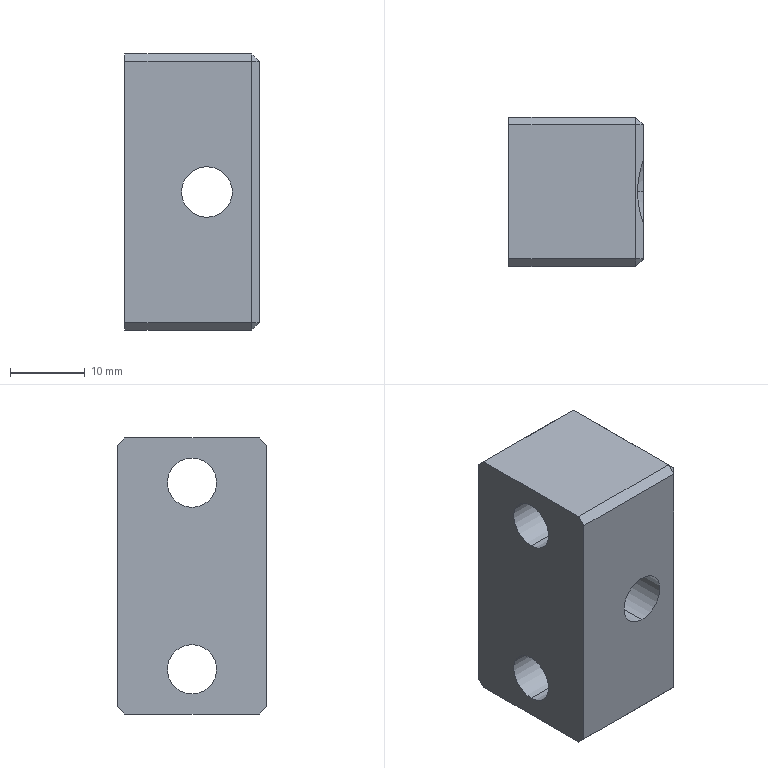Part | SolidWorks | features BaseBody 1 | 1 solid | 34 faces | box 18 x 20 x 37 mm | volume 9780 mm3 | plane 20 | cylinder 10 | cone 4 | commonest cylinder face diameters 6.6 x4 11 x4 6.8 x2
STEP:
#1=CARTESIAN_POINT('',(104.247,1826.,-338.8));
#2=VERTEX_POINT('',#1);
#3=CARTESIAN_POINT('',(104.247,1826.,-332.2));
#4=VERTEX_POINT('',#3);
#5=CARTESIAN_POINT('',(104.247,1826.,-335.5));
#6=DIRECTION('',(-1.,0.,0.));
#7=DIRECTION('',(0.,0.,-1.));
#8=AXIS2_PLACEMENT_3D('',#5,#6,#7);
#9=CIRCLE('',#8,3.3);
#10=EDGE_CURVE('',#2,#4,#9,.T.);
#11=ORIENTED_EDGE('',*,*,#10,.T.);
#12=CARTESIAN_POINT('',(110.247,1826.,-332.2));
#13=VERTEX_POINT('',#12);
#14=CARTESIAN_POINT('',(122.247,1826.,-332.2));
#15=DIRECTION('',(1.,0.,0.));
#16=VECTOR('',#15,1000.);
#17=LINE('',#14,#16);
#18=EDGE_CURVE('',#4,#13,#17,.T.);
#19=ORIENTED_EDGE('',*,*,#18,.T.);
#20=CARTESIAN_POINT('',(110.247,1826.,-338.8));
#21=VERTEX_POINT('',#20);
#22=CARTESIAN_POINT('',(110.247,1826.,-335.5));
#23=DIRECTION('',(-1.,0.,0.));
#24=DIRECTION('',(0.,0.,-1.));
#25=AXIS2_PLACEMENT_3D('',#22,#23,#24);
#26=CIRCLE('',#25,3.3);
#27=EDGE_CURVE('',#21,#13,#26,.T.);
#28=ORIENTED_EDGE('',*,*,#27,.F.);
#29=CARTESIAN_POINT('',(122.247,1826.,-338.8));
#30=DIRECTION('',(1.,0.,0.));
#31=VECTOR('',#30,1000.);
#32=LINE('',#29,#31);
#33=EDGE_CURVE('',#2,#21,#32,.T.);
#34=ORIENTED_EDGE('',*,*,#33,.F.);
#35=EDGE_LOOP('',(#11,#19,#28,#34));
#36=FACE_OUTER_BOUND('',#35,.T.);
#37=CARTESIAN_POINT('',(122.247,1826.,-335.5));
#38=DIRECTION('',(1.,0.,0.));
#39=DIRECTION('',(0.,0.,-1.));
#40=AXIS2_PLACEMENT_3D('',#37,#38,#39);
#41=CYLINDRICAL_SURFACE('',#40,3.3);
#42=ADVANCED_FACE('',(#36),#41,.F.);
#43=CARTESIAN_POINT('',(104.247,1826.,-363.8));
#44=VERTEX_POINT('',#43);
#45=CARTESIAN_POINT('',(104.247,1826.,-357.2));
#46=VERTEX_POINT('',#45);
#47=CARTESIAN_POINT('',(104.247,1826.,-360.5));
#48=DIRECTION('',(-1.,0.,0.));
#49=DIRECTION('',(0.,0.,-1.));
#50=AXIS2_PLACEMENT_3D('',#47,#48,#49);
#51=CIRCLE('',#50,3.3);
#52=EDGE_CURVE('',#44,#46,#51,.T.);
#53=ORIENTED_EDGE('',*,*,#52,.T.);
#54=CARTESIAN_POINT('',(110.247,1826.,-357.2));
#55=VERTEX_POINT('',#54);
#56=CARTESIAN_POINT('',(122.247,1826.,-357.2));
#57=DIRECTION('',(1.,0.,0.));
#58=VECTOR('',#57,1000.);
#59=LINE('',#56,#58);
#60=EDGE_CURVE('',#46,#55,#59,.T.);
#61=ORIENTED_EDGE('',*,*,#60,.T.);
#62=CARTESIAN_POINT('',(110.247,1826.,-363.8));
#63=VERTEX_POINT('',#62);
#64=CARTESIAN_POINT('',(110.247,1826.,-360.5));
#65=DIRECTION('',(-1.,0.,0.));
#66=DIRECTION('',(0.,0.,-1.));
#67=AXIS2_PLACEMENT_3D('',#64,#65,#66);
#68=CIRCLE('',#67,3.3);
#69=EDGE_CURVE('',#63,#55,#68,.T.);
#70=ORIENTED_EDGE('',*,*,#69,.F.);
#71=CARTESIAN_POINT('',(122.247,1826.,-363.8));
#72=DIRECTION('',(1.,0.,0.));
#73=VECTOR('',#72,1000.);
#74=LINE('',#71,#73);
#75=EDGE_CURVE('',#44,#63,#74,.T.);
#76=ORIENTED_EDGE('',*,*,#75,.F.);
#77=EDGE_LOOP('',(#53,#61,#70,#76));
#78=FACE_OUTER_BOUND('',#77,.T.);
#79=CARTESIAN_POINT('',(122.247,1826.,-360.5));
#80=DIRECTION('',(1.,0.,0.));
#81=DIRECTION('',(0.,0.,-1.));
#82=AXIS2_PLACEMENT_3D('',#79,#80,#81);
#83=CYLINDRICAL_SURFACE('',#82,3.3);
#84=ADVANCED_FACE('',(#78),#83,.F.);
#85=CARTESIAN_POINT('',(115.247,1836.,-351.4));
#86=VERTEX_POINT('',#85);
#87=CARTESIAN_POINT('',(115.247,1836.,-344.6));
#88=VERTEX_POINT('',#87);
#89=CARTESIAN_POINT('',(115.247,1836.,-348.));
#90=DIRECTION('',(0.,1.,0.));
#91=DIRECTION('',(0.,0.,-1.));
#92=AXIS2_PLACEMENT_3D('',#89,#90,#91);
#93=CIRCLE('',#92,3.4);
#94=EDGE_CURVE('',#86,#88,#93,.T.);
#95=ORIENTED_EDGE('',*,*,#94,.T.);
#96=CARTESIAN_POINT('',(115.247,1816.,-344.6));
#97=VERTEX_POINT('',#96);
#98=CARTESIAN_POINT('',(115.247,1816.,-344.6));
#99=DIRECTION('',(0.,-1.,0.));
#100=VECTOR('',#99,1000.);
#101=LINE('',#98,#100);
#102=EDGE_CURVE('',#88,#97,#101,.T.);
#103=ORIENTED_EDGE('',*,*,#102,.T.);
#104=CARTESIAN_POINT('',(115.247,1816.,-351.4));
#105=VERTEX_POINT('',#104);
#106=CARTESIAN_POINT('',(115.247,1816.,-348.));
#107=DIRECTION('',(0.,-1.,0.));
#108=DIRECTION('',(0.,0.,-1.));
#109=AXIS2_PLACEMENT_3D('',#106,#107,#108);
#110=CIRCLE('',#109,3.4);
#111=EDGE_CURVE('',#97,#105,#110,.T.);
#112=ORIENTED_EDGE('',*,*,#111,.T.);
#113=CARTESIAN_POINT('',(115.247,1816.,-351.4));
#114=DIRECTION('',(0.,-1.,0.));
#115=VECTOR('',#114,1000.);
#116=LINE('',#113,#115);
#117=EDGE_CURVE('',#86,#105,#116,.T.);
#118=ORIENTED_EDGE('',*,*,#117,.F.);
#119=EDGE_LOOP('',(#95,#103,#112,#118));
#120=FACE_OUTER_BOUND('',#119,.T.);
#121=CARTESIAN_POINT('',(115.247,1816.,-348.));
#122=DIRECTION('',(0.,-1.,0.));
#123=DIRECTION('',(0.,0.,-1.));
#124=AXIS2_PLACEMENT_3D('',#121,#122,#123);
#125=CYLINDRICAL_SURFACE('',#124,3.4);
#126=ADVANCED_FACE('',(#120),#125,.F.);
#127=CARTESIAN_POINT('',(110.247,1826.,-341.));
#128=VERTEX_POINT('',#127);
#129=CARTESIAN_POINT('',(110.247,1826.,-330.));
#130=VERTEX_POINT('',#129);
#131=CARTESIAN_POINT('',(110.247,1826.,-335.5));
#132=DIRECTION('',(-1.,0.,0.));
#133=DIRECTION('',(0.,0.,-1.));
#134=AXIS2_PLACEMENT_3D('',#131,#132,#133);
#135=CIRCLE('',#134,5.5);
#136=EDGE_CURVE('',#128,#130,#135,.T.);
#137=ORIENTED_EDGE('',*,*,#136,.T.);
#138=CARTESIAN_POINT('',(121.247,1826.,-330.));
#139=VERTEX_POINT('',#138);
#140=CARTESIAN_POINT('',(122.247,1826.,-330.));
#141=DIRECTION('',(1.,0.,0.));
#142=VECTOR('',#141,1000.);
#143=LINE('',#140,#142);
#144=EDGE_CURVE('',#130,#139,#143,.T.);
#145=ORIENTED_EDGE('',*,*,#144,.T.);
#146=CARTESIAN_POINT('',(121.247,1826.,-341.));
#147=VERTEX_POINT('',#146);
#148=CARTESIAN_POINT('',(121.247,1826.,-335.5));
#149=DIRECTION('',(-1.,0.,0.));
#150=DIRECTION('',(0.,0.,-1.));
#151=AXIS2_PLACEMENT_3D('',#148,#149,#150);
#152=CIRCLE('',#151,5.5);
#153=EDGE_CURVE('',#147,#139,#152,.T.);
#154=ORIENTED_EDGE('',*,*,#153,.F.);
#155=CARTESIAN_POINT('',(122.247,1826.,-341.));
#156=DIRECTION('',(1.,0.,0.));
#157=VECTOR('',#156,1000.);
#158=LINE('',#155,#157);
#159=EDGE_CURVE('',#128,#147,#158,.T.);
#160=ORIENTED_EDGE('',*,*,#159,.F.);
#161=EDGE_LOOP('',(#137,#145,#154,#160));
#162=FACE_OUTER_BOUND('',#161,.T.);
#163=CARTESIAN_POINT('',(122.247,1826.,-335.5));
#164=DIRECTION('',(1.,0.,0.));
#165=DIRECTION('',(0.,0.,-1.));
#166=AXIS2_PLACEMENT_3D('',#163,#164,#165);
#167=CYLINDRICAL_SURFACE('',#166,5.5);
#168=ADVANCED_FACE('',(#162),#167,.F.);
#169=CARTESIAN_POINT('',(110.247,1826.,-366.));
#170=VERTEX_POINT('',#169);
#171=CARTESIAN_POINT('',(110.247,1826.,-355.));
#172=VERTEX_POINT('',#171);
#173=CARTESIAN_POINT('',(110.247,1826.,-360.5));
#174=DIRECTION('',(-1.,0.,0.));
#175=DIRECTION('',(0.,0.,-1.));
#176=AXIS2_PLACEMENT_3D('',#173,#174,#175);
#177=CIRCLE('',#176,5.5);
#178=EDGE_CURVE('',#170,#172,#177,.T.);
#179=ORIENTED_EDGE('',*,*,#178,.T.);
#180=CARTESIAN_POINT('',(121.247,1826.,-355.));
#181=VERTEX_POINT('',#180);
#182=CARTESIAN_POINT('',(122.247,1826.,-355.));
#183=DIRECTION('',(1.,0.,0.));
#184=VECTOR('',#183,1000.);
#185=LINE('',#182,#184);
#186=EDGE_CURVE('',#172,#181,#185,.T.);
#187=ORIENTED_EDGE('',*,*,#186,.T.);
#188=CARTESIAN_POINT('',(121.247,1826.,-366.));
#189=VERTEX_POINT('',#188);
#190=CARTESIAN_POINT('',(121.247,1826.,-360.5));
#191=DIRECTION('',(-1.,0.,0.));
#192=DIRECTION('',(0.,0.,-1.));
#193=AXIS2_PLACEMENT_3D('',#190,#191,#192);
#194=CIRCLE('',#193,5.5);
#195=EDGE_CURVE('',#189,#181,#194,.T.);
#196=ORIENTED_EDGE('',*,*,#195,.F.);
#197=CARTESIAN_POINT('',(122.247,1826.,-366.));
#198=DIRECTION('',(1.,0.,0.));
#199=VECTOR('',#198,1000.);
#200=LINE('',#197,#199);
#201=EDGE_CURVE('',#170,#189,#200,.T.);
#202=ORIENTED_EDGE('',*,*,#201,.F.);
#203=EDGE_LOOP('',(#179,#187,#196,#202));
#204=FACE_OUTER_BOUND('',#203,.T.);
#205=CARTESIAN_POINT('',(122.247,1826.,-360.5));
#206=DIRECTION('',(1.,0.,0.));
#207=DIRECTION('',(0.,0.,-1.));
#208=AXIS2_PLACEMENT_3D('',#205,#206,#207);
#209=CYLINDRICAL_SURFACE('',#208,5.5);
#210=ADVANCED_FACE('',(#204),#209,.F.);
#211=ORIENTED_EDGE('',*,*,#153,.T.);
#212=CARTESIAN_POINT('',(121.497,1826.,-329.75));
#213=VERTEX_POINT('',#212);
#214=CARTESIAN_POINT('',(122.247,1826.,-329.));
#215=DIRECTION('',(0.7071,0.,0.7071));
#216=VECTOR('',#215,1000.);
#217=LINE('',#214,#216);
#218=EDGE_CURVE('',#139,#213,#217,.T.);
#219=ORIENTED_EDGE('',*,*,#218,.T.);
#220=CARTESIAN_POINT('',(122.247,1821.847,-330.5));
#221=VERTEX_POINT('',#220);
#222=CARTESIAN_POINT('',(122.247,1821.847,-330.5));
#223=CARTESIAN_POINT('',(121.747,1823.231,-330.));
#224=CARTESIAN_POINT('',(121.497,1824.616,-329.75));
#225=CARTESIAN_POINT('',(121.497,1826.,-329.75));
#226=B_SPLINE_CURVE_WITH_KNOTS('',3,(#222,#223,#224,#225),.UNSPECIFIED.,.F.,.F.,(4,4),(0.,0.5),.UNSPECIFIED.);
#227=EDGE_CURVE('',#221,#213,#226,.T.);
#228=ORIENTED_EDGE('',*,*,#227,.F.);
#229=CARTESIAN_POINT('',(122.247,1826.,-342.));
#230=VERTEX_POINT('',#229);
#231=CARTESIAN_POINT('',(122.247,1826.,-335.5));
#232=DIRECTION('',(-1.,0.,0.));
#233=DIRECTION('',(0.,0.,-1.));
#234=AXIS2_PLACEMENT_3D('',#231,#232,#233);
#235=CIRCLE('',#234,6.5);
#236=EDGE_CURVE('',#230,#221,#235,.T.);
#237=ORIENTED_EDGE('',*,*,#236,.F.);
#238=CARTESIAN_POINT('',(122.247,1826.,-342.));
#239=DIRECTION('',(0.7071,0.,-0.7071));
#240=VECTOR('',#239,1000.);
#241=LINE('',#238,#240);
#242=EDGE_CURVE('',#147,#230,#241,.T.);
#243=ORIENTED_EDGE('',*,*,#242,.F.);
#244=EDGE_LOOP('',(#211,#219,#228,#237,#243));
#245=FACE_OUTER_BOUND('',#244,.T.);
#246=CARTESIAN_POINT('',(122.247,1826.,-335.5));
#247=DIRECTION('',(1.,0.,0.));
#248=DIRECTION('',(0.,0.,-1.));
#249=AXIS2_PLACEMENT_3D('',#246,#247,#248);
#250=CONICAL_SURFACE('',#249,6.5,0.7854);
#251=ADVANCED_FACE('',(#245),#250,.F.);
#252=ORIENTED_EDGE('',*,*,#195,.T.);
#253=CARTESIAN_POINT('',(122.247,1826.,-354.));
#254=VERTEX_POINT('',#253);
#255=CARTESIAN_POINT('',(122.247,1826.,-354.));
#256=DIRECTION('',(0.7071,0.,0.7071));
#257=VECTOR('',#256,1000.);
#258=LINE('',#255,#257);
#259=EDGE_CURVE('',#181,#254,#258,.T.);
#260=ORIENTED_EDGE('',*,*,#259,.T.);
#261=CARTESIAN_POINT('',(122.247,1821.847,-365.5));
#262=VERTEX_POINT('',#261);
#263=CARTESIAN_POINT('',(122.247,1826.,-360.5));
#264=DIRECTION('',(-1.,0.,0.));
#265=DIRECTION('',(0.,0.,-1.));
#266=AXIS2_PLACEMENT_3D('',#263,#264,#265);
#267=CIRCLE('',#266,6.5);
#268=EDGE_CURVE('',#262,#254,#267,.T.);
#269=ORIENTED_EDGE('',*,*,#268,.F.);
#270=CARTESIAN_POINT('',(121.497,1826.,-366.25));
#271=VERTEX_POINT('',#270);
#272=CARTESIAN_POINT('',(121.497,1826.,-366.25));
#273=CARTESIAN_POINT('',(121.497,1824.616,-366.25));
#274=CARTESIAN_POINT('',(121.747,1823.231,-366.));
#275=CARTESIAN_POINT('',(122.247,1821.847,-365.5));
#276=B_SPLINE_CURVE_WITH_KNOTS('',3,(#272,#273,#274,#275),.UNSPECIFIED.,.F.,.F.,(4,4),(0.5,1.),.UNSPECIFIED.);
#277=EDGE_CURVE('',#271,#262,#276,.T.);
#278=ORIENTED_EDGE('',*,*,#277,.F.);
#279=CARTESIAN_POINT('',(122.247,1826.,-367.));
#280=DIRECTION('',(0.7071,0.,-0.7071));
#281=VECTOR('',#280,1000.);
#282=LINE('',#279,#281);
#283=EDGE_CURVE('',#189,#271,#282,.T.);
#284=ORIENTED_EDGE('',*,*,#283,.F.);
#285=EDGE_LOOP('',(#252,#260,#269,#278,#284));
#286=FACE_OUTER_BOUND('',#285,.T.);
#287=CARTESIAN_POINT('',(122.247,1826.,-360.5));
#288=DIRECTION('',(1.,0.,0.));
#289=DIRECTION('',(0.,0.,-1.));
#290=AXIS2_PLACEMENT_3D('',#287,#288,#289);
#291=CONICAL_SURFACE('',#290,6.5,0.7854);
#292=ADVANCED_FACE('',(#286),#291,.F.);
#293=ORIENTED_EDGE('',*,*,#10,.F.);
#294=CARTESIAN_POINT('',(104.247,1826.,-335.5));
#295=DIRECTION('',(-1.,0.,0.));
#296=DIRECTION('',(0.,0.,-1.));
#297=AXIS2_PLACEMENT_3D('',#294,#295,#296);
#298=CIRCLE('',#297,3.3);
#299=EDGE_CURVE('',#4,#2,#298,.T.);
#300=ORIENTED_EDGE('',*,*,#299,.F.);
#301=EDGE_LOOP('',(#293,#300));
#302=FACE_BOUND('',#301,.T.);
#303=ORIENTED_EDGE('',*,*,#52,.F.);
#304=CARTESIAN_POINT('',(104.247,1826.,-360.5));
#305=DIRECTION('',(-1.,0.,0.));
#306=DIRECTION('',(0.,0.,-1.));
#307=AXIS2_PLACEMENT_3D('',#304,#305,#306);
#308=CIRCLE('',#307,3.3);
#309=EDGE_CURVE('',#46,#44,#308,.T.);
#310=ORIENTED_EDGE('',*,*,#309,.F.);
#311=EDGE_LOOP('',(#303,#310));
#312=FACE_BOUND('',#311,.T.);
#313=CARTESIAN_POINT('',(104.247,1816.,-330.5));
#314=VERTEX_POINT('',#313);
#315=CARTESIAN_POINT('',(104.247,1816.,-365.5));
#316=VERTEX_POINT('',#315);
#317=CARTESIAN_POINT('',(104.247,1816.,-348.));
#318=DIRECTION('',(0.,0.,-1.));
#319=VECTOR('',#318,1000.);
#320=LINE('',#317,#319);
#321=EDGE_CURVE('',#314,#316,#320,.T.);
#322=ORIENTED_EDGE('',*,*,#321,.F.);
#323=CARTESIAN_POINT('',(104.247,1817.,-329.5));
#324=VERTEX_POINT('',#323);
#325=CARTESIAN_POINT('',(104.247,1817.,-329.5));
#326=DIRECTION('',(0.,-0.7071,-0.7071));
#327=VECTOR('',#326,1000.);
#328=LINE('',#325,#327);
#329=EDGE_CURVE('',#324,#314,#328,.T.);
#330=ORIENTED_EDGE('',*,*,#329,.F.);
#331=CARTESIAN_POINT('',(104.247,1835.,-329.5));
#332=VERTEX_POINT('',#331);
#333=CARTESIAN_POINT('',(104.247,1826.,-329.5));
#334=DIRECTION('',(0.,-1.,0.));
#335=VECTOR('',#334,1000.);
#336=LINE('',#333,#335);
#337=EDGE_CURVE('',#332,#324,#336,.T.);
#338=ORIENTED_EDGE('',*,*,#337,.F.);
#339=CARTESIAN_POINT('',(104.247,1836.,-330.5));
#340=VERTEX_POINT('',#339);
#341=CARTESIAN_POINT('',(104.247,1836.,-330.5));
#342=DIRECTION('',(0.,-0.7071,0.7071));
#343=VECTOR('',#342,1000.);
#344=LINE('',#341,#343);
#345=EDGE_CURVE('',#340,#332,#344,.T.);
#346=ORIENTED_EDGE('',*,*,#345,.F.);
#347=CARTESIAN_POINT('',(104.247,1836.,-365.5));
#348=VERTEX_POINT('',#347);
#349=CARTESIAN_POINT('',(104.247,1836.,-348.));
#350=DIRECTION('',(0.,0.,1.));
#351=VECTOR('',#350,1000.);
#352=LINE('',#349,#351);
#353=EDGE_CURVE('',#348,#340,#352,.T.);
#354=ORIENTED_EDGE('',*,*,#353,.F.);
#355=CARTESIAN_POINT('',(104.247,1835.,-366.5));
#356=VERTEX_POINT('',#355);
#357=CARTESIAN_POINT('',(104.247,1835.,-366.5));
#358=DIRECTION('',(0.,0.7071,0.7071));
#359=VECTOR('',#358,1000.);
#360=LINE('',#357,#359);
#361=EDGE_CURVE('',#356,#348,#360,.T.);
#362=ORIENTED_EDGE('',*,*,#361,.F.);
#363=CARTESIAN_POINT('',(104.247,1817.,-366.5));
#364=VERTEX_POINT('',#363);
#365=CARTESIAN_POINT('',(104.247,1826.,-366.5));
#366=DIRECTION('',(0.,1.,0.));
#367=VECTOR('',#366,1000.);
#368=LINE('',#365,#367);
#369=EDGE_CURVE('',#364,#356,#368,.T.);
#370=ORIENTED_EDGE('',*,*,#369,.F.);
#371=CARTESIAN_POINT('',(104.247,1816.,-365.5));
#372=DIRECTION('',(0.,0.7071,-0.7071));
#373=VECTOR('',#372,1000.);
#374=LINE('',#371,#373);
#375=EDGE_CURVE('',#316,#364,#374,.T.);
#376=ORIENTED_EDGE('',*,*,#375,.F.);
#377=EDGE_LOOP('',(#322,#330,#338,#346,#354,#362,#370,#376));
#378=FACE_OUTER_BOUND('',#377,.T.);
#379=CARTESIAN_POINT('',(104.247,1826.,-348.));
#380=DIRECTION('',(1.,0.,0.));
#381=DIRECTION('',(0.,0.,-1.));
#382=AXIS2_PLACEMENT_3D('',#379,#380,#381);
#383=PLANE('',#382);
#384=ADVANCED_FACE('',(#302,#312,#378),#383,.F.);
#385=ORIENTED_EDGE('',*,*,#18,.F.);
#386=ORIENTED_EDGE('',*,*,#299,.T.);
#387=ORIENTED_EDGE('',*,*,#33,.T.);
#388=CARTESIAN_POINT('',(110.247,1826.,-335.5));
#389=DIRECTION('',(-1.,0.,0.));
#390=DIRECTION('',(0.,0.,-1.));
#391=AXIS2_PLACEMENT_3D('',#388,#389,#390);
#392=CIRCLE('',#391,3.3);
#393=EDGE_CURVE('',#13,#21,#392,.T.);
#394=ORIENTED_EDGE('',*,*,#393,.F.);
#395=EDGE_LOOP('',(#385,#386,#387,#394));
#396=FACE_OUTER_BOUND('',#395,.T.);
#397=CARTESIAN_POINT('',(122.247,1826.,-335.5));
#398=DIRECTION('',(1.,0.,0.));
#399=DIRECTION('',(0.,0.,-1.));
#400=AXIS2_PLACEMENT_3D('',#397,#398,#399);
#401=CYLINDRICAL_SURFACE('',#400,3.3);
#402=ADVANCED_FACE('',(#396),#401,.F.);
#403=ORIENTED_EDGE('',*,*,#60,.F.);
#404=ORIENTED_EDGE('',*,*,#309,.T.);
#405=ORIENTED_EDGE('',*,*,#75,.T.);
#406=CARTESIAN_POINT('',(110.247,1826.,-360.5));
#407=DIRECTION('',(-1.,0.,0.));
#408=DIRECTION('',(0.,0.,-1.));
#409=AXIS2_PLACEMENT_3D('',#406,#407,#408);
#410=CIRCLE('',#409,3.3);
#411=EDGE_CURVE('',#55,#63,#410,.T.);
#412=ORIENTED_EDGE('',*,*,#411,.F.);
#413=EDGE_LOOP('',(#403,#404,#405,#412));
#414=FACE_OUTER_BOUND('',#413,.T.);
#415=CARTESIAN_POINT('',(122.247,1826.,-360.5));
#416=DIRECTION('',(1.,0.,0.));
#417=DIRECTION('',(0.,0.,-1.));
#418=AXIS2_PLACEMENT_3D('',#415,#416,#417);
#419=CYLINDRICAL_SURFACE('',#418,3.3);
#420=ADVANCED_FACE('',(#414),#419,.F.);
#421=CARTESIAN_POINT('',(121.247,1816.,-365.5));
#422=VERTEX_POINT('',#421);
#423=CARTESIAN_POINT('',(121.247,1817.,-366.5));
#424=VERTEX_POINT('',#423);
#425=CARTESIAN_POINT('',(121.247,1817.,-366.5));
#426=DIRECTION('',(0.,0.7071,-0.7071));
#427=VECTOR('',#426,1000.);
#428=LINE('',#425,#427);
#429=EDGE_CURVE('',#422,#424,#428,.T.);
#430=ORIENTED_EDGE('',*,*,#429,.F.);
#431=CARTESIAN_POINT('',(122.247,1816.,-365.5));
#432=DIRECTION('',(1.,0.,0.));
#433=VECTOR('',#432,1000.);
#434=LINE('',#431,#433);
#435=EDGE_CURVE('',#316,#422,#434,.T.);
#436=ORIENTED_EDGE('',*,*,#435,.F.);
#437=ORIENTED_EDGE('',*,*,#375,.T.);
#438=CARTESIAN_POINT('',(122.247,1817.,-366.5));
#439=DIRECTION('',(-1.,0.,0.));
#440=VECTOR('',#439,1000.);
#441=LINE('',#438,#440);
#442=EDGE_CURVE('',#424,#364,#441,.T.);
#443=ORIENTED_EDGE('',*,*,#442,.F.);
#444=EDGE_LOOP('',(#430,#436,#437,#443));
#445=FACE_OUTER_BOUND('',#444,.T.);
#446=CARTESIAN_POINT('',(122.247,1817.,-366.5));
#447=DIRECTION('',(0.,0.7071,0.7071));
#448=DIRECTION('',(0.,-0.7071,0.7071));
#449=AXIS2_PLACEMENT_3D('',#446,#447,#448);
#450=PLANE('',#449);
#451=ADVANCED_FACE('',(#445),#450,.F.);
#452=CARTESIAN_POINT('',(115.247,1816.,-348.));
#453=DIRECTION('',(0.,-1.,0.));
#454=DIRECTION('',(0.,0.,-1.));
#455=AXIS2_PLACEMENT_3D('',#452,#453,#454);
#456=CIRCLE('',#455,3.4);
#457=EDGE_CURVE('',#105,#97,#456,.T.);
#458=ORIENTED_EDGE('',*,*,#457,.F.);
#459=ORIENTED_EDGE('',*,*,#111,.F.);
#460=EDGE_LOOP('',(#458,#459));
#461=FACE_BOUND('',#460,.T.);
#462=CARTESIAN_POINT('',(121.247,1816.,-330.5));
#463=VERTEX_POINT('',#462);
#464=CARTESIAN_POINT('',(121.247,1816.,-329.5));
#465=DIRECTION('',(0.,0.,-1.));
#466=VECTOR('',#465,1000.);
#467=LINE('',#464,#466);
#468=EDGE_CURVE('',#463,#422,#467,.T.);
#469=ORIENTED_EDGE('',*,*,#468,.F.);
#470=CARTESIAN_POINT('',(122.247,1816.,-330.5));
#471=DIRECTION('',(1.,0.,0.));
#472=VECTOR('',#471,1000.);
#473=LINE('',#470,#472);
#474=EDGE_CURVE('',#314,#463,#473,.T.);
#475=ORIENTED_EDGE('',*,*,#474,.F.);
#476=ORIENTED_EDGE('',*,*,#321,.T.);
#477=ORIENTED_EDGE('',*,*,#435,.T.);
#478=EDGE_LOOP('',(#469,#475,#476,#477));
#479=FACE_OUTER_BOUND('',#478,.T.);
#480=CARTESIAN_POINT('',(122.247,1816.,-329.5));
#481=DIRECTION('',(0.,1.,0.));
#482=DIRECTION('',(0.,0.,1.));
#483=AXIS2_PLACEMENT_3D('',#480,#481,#482);
#484=PLANE('',#483);
#485=ADVANCED_FACE('',(#461,#479),#484,.F.);
#486=CARTESIAN_POINT('',(121.247,1817.,-329.5));
#487=VERTEX_POINT('',#486);
#488=CARTESIAN_POINT('',(121.247,1816.,-330.5));
#489=DIRECTION('',(0.,-0.7071,-0.7071));
#490=VECTOR('',#489,1000.);
#491=LINE('',#488,#490);
#492=EDGE_CURVE('',#487,#463,#491,.T.);
#493=ORIENTED_EDGE('',*,*,#492,.F.);
#494=CARTESIAN_POINT('',(122.247,1817.,-329.5));
#495=DIRECTION('',(1.,0.,0.));
#496=VECTOR('',#495,1000.);
#497=LINE('',#494,#496);
#498=EDGE_CURVE('',#324,#487,#497,.T.);
#499=ORIENTED_EDGE('',*,*,#498,.F.);
#500=ORIENTED_EDGE('',*,*,#329,.T.);
#501=ORIENTED_EDGE('',*,*,#474,.T.);
#502=EDGE_LOOP('',(#493,#499,#500,#501));
#503=FACE_OUTER_BOUND('',#502,.T.);
#504=CARTESIAN_POINT('',(122.247,1816.,-330.5));
#505=DIRECTION('',(0.,0.7071,-0.7071));
#506=DIRECTION('',(0.,0.7071,0.7071));
#507=AXIS2_PLACEMENT_3D('',#504,#505,#506);
#508=PLANE('',#507);
#509=ADVANCED_FACE('',(#503),#508,.F.);
#510=ORIENTED_EDGE('',*,*,#337,.T.);
#511=ORIENTED_EDGE('',*,*,#498,.T.);
#512=CARTESIAN_POINT('',(121.247,1835.,-329.5));
#513=VERTEX_POINT('',#512);
#514=CARTESIAN_POINT('',(121.247,1816.,-329.5));
#515=DIRECTION('',(0.,-1.,0.));
#516=VECTOR('',#515,1000.);
#517=LINE('',#514,#516);
#518=EDGE_CURVE('',#513,#487,#517,.T.);
#519=ORIENTED_EDGE('',*,*,#518,.F.);
#520=CARTESIAN_POINT('',(122.247,1835.,-329.5));
#521=DIRECTION('',(1.,0.,0.));
#522=VECTOR('',#521,1000.);
#523=LINE('',#520,#522);
#524=EDGE_CURVE('',#332,#513,#523,.T.);
#525=ORIENTED_EDGE('',*,*,#524,.F.);
#526=EDGE_LOOP('',(#510,#511,#519,#525));
#527=FACE_OUTER_BOUND('',#526,.T.);
#528=CARTESIAN_POINT('',(122.247,1816.,-329.5));
#529=DIRECTION('',(0.,0.,-1.));
#530=DIRECTION('',(-1.,0.,0.));
#531=AXIS2_PLACEMENT_3D('',#528,#529,#530);
#532=PLANE('',#531);
#533=ADVANCED_FACE('',(#527),#532,.F.);
#534=CARTESIAN_POINT('',(121.247,1836.,-330.5));
#535=VERTEX_POINT('',#534);
#536=CARTESIAN_POINT('',(121.247,1835.,-329.5));
#537=DIRECTION('',(0.,-0.7071,0.7071));
#538=VECTOR('',#537,1000.);
#539=LINE('',#536,#538);
#540=EDGE_CURVE('',#535,#513,#539,.T.);
#541=ORIENTED_EDGE('',*,*,#540,.F.);
#542=CARTESIAN_POINT('',(122.247,1836.,-330.5));
#543=DIRECTION('',(1.,0.,0.));
#544=VECTOR('',#543,1000.);
#545=LINE('',#542,#544);
#546=EDGE_CURVE('',#340,#535,#545,.T.);
#547=ORIENTED_EDGE('',*,*,#546,.F.);
#548=ORIENTED_EDGE('',*,*,#345,.T.);
#549=ORIENTED_EDGE('',*,*,#524,.T.);
#550=EDGE_LOOP('',(#541,#547,#548,#549));
#551=FACE_OUTER_BOUND('',#550,.T.);
#552=CARTESIAN_POINT('',(122.247,1835.,-329.5));
#553=DIRECTION('',(0.,-0.7071,-0.7071));
#554=DIRECTION('',(0.,0.7071,-0.7071));
#555=AXIS2_PLACEMENT_3D('',#552,#553,#554);
#556=PLANE('',#555);
#557=ADVANCED_FACE('',(#551),#556,.F.);
#558=ORIENTED_EDGE('',*,*,#94,.F.);
#559=CARTESIAN_POINT('',(115.247,1836.,-348.));
#560=DIRECTION('',(0.,1.,0.));
#561=DIRECTION('',(0.,0.,-1.));
#562=AXIS2_PLACEMENT_3D('',#559,#560,#561);
#563=CIRCLE('',#562,3.4);
#564=EDGE_CURVE('',#88,#86,#563,.T.);
#565=ORIENTED_EDGE('',*,*,#564,.F.);
#566=EDGE_LOOP('',(#558,#565));
#567=FACE_BOUND('',#566,.T.);
#568=ORIENTED_EDGE('',*,*,#353,.T.);
#569=ORIENTED_EDGE('',*,*,#546,.T.);
#570=CARTESIAN_POINT('',(121.247,1836.,-365.5));
#571=VERTEX_POINT('',#570);
#572=CARTESIAN_POINT('',(121.247,1836.,-329.5));
#573=DIRECTION('',(0.,0.,1.));
#574=VECTOR('',#573,1000.);
#575=LINE('',#572,#574);
#576=EDGE_CURVE('',#571,#535,#575,.T.);
#577=ORIENTED_EDGE('',*,*,#576,.F.);
#578=CARTESIAN_POINT('',(122.247,1836.,-365.5));
#579=DIRECTION('',(1.,0.,0.));
#580=VECTOR('',#579,1000.);
#581=LINE('',#578,#580);
#582=EDGE_CURVE('',#348,#571,#581,.T.);
#583=ORIENTED_EDGE('',*,*,#582,.F.);
#584=EDGE_LOOP('',(#568,#569,#577,#583));
#585=FACE_OUTER_BOUND('',#584,.T.);
#586=CARTESIAN_POINT('',(122.247,1836.,-329.5));
#587=DIRECTION('',(0.,-1.,0.));
#588=DIRECTION('',(0.,0.,-1.));
#589=AXIS2_PLACEMENT_3D('',#586,#587,#588);
#590=PLANE('',#589);
#591=ADVANCED_FACE('',(#567,#585),#590,.F.);
#592=CARTESIAN_POINT('',(121.247,1835.,-366.5));
#593=VERTEX_POINT('',#592);
#594=CARTESIAN_POINT('',(121.247,1836.,-365.5));
#595=DIRECTION('',(0.,0.7071,0.7071));
#596=VECTOR('',#595,1000.);
#597=LINE('',#594,#596);
#598=EDGE_CURVE('',#593,#571,#597,.T.);
#599=ORIENTED_EDGE('',*,*,#598,.F.);
#600=CARTESIAN_POINT('',(122.247,1835.,-366.5));
#601=DIRECTION('',(1.,0.,0.));
#602=VECTOR('',#601,1000.);
#603=LINE('',#600,#602);
#604=EDGE_CURVE('',#356,#593,#603,.T.);
#605=ORIENTED_EDGE('',*,*,#604,.F.);
#606=ORIENTED_EDGE('',*,*,#361,.T.);
#607=ORIENTED_EDGE('',*,*,#582,.T.);
#608=EDGE_LOOP('',(#599,#605,#606,#607));
#609=FACE_OUTER_BOUND('',#608,.T.);
#610=CARTESIAN_POINT('',(122.247,1836.,-365.5));
#611=DIRECTION('',(0.,-0.7071,0.7071));
#612=DIRECTION('',(0.,-0.7071,-0.7071));
#613=AXIS2_PLACEMENT_3D('',#610,#611,#612);
#614=PLANE('',#613);
#615=ADVANCED_FACE('',(#609),#614,.F.);
#616=ORIENTED_EDGE('',*,*,#369,.T.);
#617=ORIENTED_EDGE('',*,*,#604,.T.);
#618=CARTESIAN_POINT('',(121.247,1816.,-366.5));
#619=DIRECTION('',(0.,1.,0.));
#620=VECTOR('',#619,1000.);
#621=LINE('',#618,#620);
#622=EDGE_CURVE('',#424,#593,#621,.T.);
#623=ORIENTED_EDGE('',*,*,#622,.F.);
#624=ORIENTED_EDGE('',*,*,#442,.T.);
#625=EDGE_LOOP('',(#616,#617,#623,#624));
#626=FACE_OUTER_BOUND('',#625,.T.);
#627=CARTESIAN_POINT('',(122.247,1816.,-366.5));
#628=DIRECTION('',(0.,0.,1.));
#629=DIRECTION('',(1.,0.,0.));
#630=AXIS2_PLACEMENT_3D('',#627,#628,#629);
#631=PLANE('',#630);
#632=ADVANCED_FACE('',(#626),#631,.F.);
#633=ORIENTED_EDGE('',*,*,#27,.T.);
#634=ORIENTED_EDGE('',*,*,#393,.T.);
#635=EDGE_LOOP('',(#633,#634));
#636=FACE_BOUND('',#635,.T.);
#637=ORIENTED_EDGE('',*,*,#136,.F.);
#638=CARTESIAN_POINT('',(110.247,1826.,-335.5));
#639=DIRECTION('',(-1.,0.,0.));
#640=DIRECTION('',(0.,0.,-1.));
#641=AXIS2_PLACEMENT_3D('',#638,#639,#640);
#642=CIRCLE('',#641,5.5);
#643=EDGE_CURVE('',#130,#128,#642,.T.);
#644=ORIENTED_EDGE('',*,*,#643,.F.);
#645=EDGE_LOOP('',(#637,#644));
#646=FACE_OUTER_BOUND('',#645,.T.);
#647=CARTESIAN_POINT('',(110.247,1826.,-332.2));
#648=DIRECTION('',(-1.,0.,0.));
#649=DIRECTION('',(0.,0.,1.));
#650=AXIS2_PLACEMENT_3D('',#647,#648,#649);
#651=PLANE('',#650);
#652=ADVANCED_FACE('',(#636,#646),#651,.F.);
#653=ORIENTED_EDGE('',*,*,#69,.T.);
#654=ORIENTED_EDGE('',*,*,#411,.T.);
#655=EDGE_LOOP('',(#653,#654));
#656=FACE_BOUND('',#655,.T.);
#657=ORIENTED_EDGE('',*,*,#178,.F.);
#658=CARTESIAN_POINT('',(110.247,1826.,-360.5));
#659=DIRECTION('',(-1.,0.,0.));
#660=DIRECTION('',(0.,0.,-1.));
#661=AXIS2_PLACEMENT_3D('',#658,#659,#660);
#662=CIRCLE('',#661,5.5);
#663=EDGE_CURVE('',#172,#170,#662,.T.);
#664=ORIENTED_EDGE('',*,*,#663,.F.);
#665=EDGE_LOOP('',(#657,#664));
#666=FACE_OUTER_BOUND('',#665,.T.);
#667=CARTESIAN_POINT('',(110.247,1826.,-357.2));
#668=DIRECTION('',(-1.,0.,0.));
#669=DIRECTION('',(0.,0.,1.));
#670=AXIS2_PLACEMENT_3D('',#667,#668,#669);
#671=PLANE('',#670);
#672=ADVANCED_FACE('',(#656,#666),#671,.F.);
#673=CARTESIAN_POINT('',(122.247,1817.,-365.5));
#674=VERTEX_POINT('',#673);
#675=CARTESIAN_POINT('',(121.247,1817.,-366.5));
#676=DIRECTION('',(0.7071,0.,0.7071));
#677=VECTOR('',#676,1000.);
#678=LINE('',#675,#677);
#679=EDGE_CURVE('',#424,#674,#678,.T.);
#680=ORIENTED_EDGE('',*,*,#679,.T.);
#681=CARTESIAN_POINT('',(122.247,1817.,-365.5));
#682=DIRECTION('',(-0.7071,-0.7071,0.));
#683=VECTOR('',#682,1000.);
#684=LINE('',#681,#683);
#685=EDGE_CURVE('',#674,#422,#684,.T.);
#686=ORIENTED_EDGE('',*,*,#685,.T.);
#687=ORIENTED_EDGE('',*,*,#429,.T.);
#688=EDGE_LOOP('',(#680,#686,#687));
#689=FACE_OUTER_BOUND('',#688,.T.);
#690=CARTESIAN_POINT('',(121.247,1817.,-366.5));
#691=DIRECTION('',(0.5774,-0.5774,-0.5774));
#692=DIRECTION('',(-0.7071,0.,-0.7071));
#693=AXIS2_PLACEMENT_3D('',#690,#691,#692);
#694=PLANE('',#693);
#695=ADVANCED_FACE('',(#689),#694,.T.);
#696=ORIENTED_EDGE('',*,*,#102,.F.);
#697=ORIENTED_EDGE('',*,*,#564,.T.);
#698=ORIENTED_EDGE('',*,*,#117,.T.);
#699=ORIENTED_EDGE('',*,*,#457,.T.);
#700=EDGE_LOOP('',(#696,#697,#698,#699));
#701=FACE_OUTER_BOUND('',#700,.T.);
#702=CARTESIAN_POINT('',(115.247,1816.,-348.));
#703=DIRECTION('',(0.,-1.,0.));
#704=DIRECTION('',(0.,0.,-1.));
#705=AXIS2_PLACEMENT_3D('',#702,#703,#704);
#706=CYLINDRICAL_SURFACE('',#705,3.4);
#707=ADVANCED_FACE('',(#701),#706,.F.);
#708=CARTESIAN_POINT('',(122.247,1817.,-330.5));
#709=VERTEX_POINT('',#708);
#710=CARTESIAN_POINT('',(122.247,1817.,-348.));
#711=DIRECTION('',(0.,0.,1.));
#712=VECTOR('',#711,1000.);
#713=LINE('',#710,#712);
#714=EDGE_CURVE('',#674,#709,#713,.T.);
#715=ORIENTED_EDGE('',*,*,#714,.T.);
#716=CARTESIAN_POINT('',(122.247,1817.,-330.5));
#717=DIRECTION('',(-0.7071,-0.7071,0.));
#718=VECTOR('',#717,1000.);
#719=LINE('',#716,#718);
#720=EDGE_CURVE('',#709,#463,#719,.T.);
#721=ORIENTED_EDGE('',*,*,#720,.T.);
#722=ORIENTED_EDGE('',*,*,#468,.T.);
#723=ORIENTED_EDGE('',*,*,#685,.F.);
#724=EDGE_LOOP('',(#715,#721,#722,#723));
#725=FACE_OUTER_BOUND('',#724,.T.);
#726=CARTESIAN_POINT('',(122.247,1817.,-348.));
#727=DIRECTION('',(0.7071,-0.7071,0.));
#728=DIRECTION('',(0.7071,0.7071,0.));
#729=AXIS2_PLACEMENT_3D('',#726,#727,#728);
#730=PLANE('',#729);
#731=ADVANCED_FACE('',(#725),#730,.T.);
#732=ORIENTED_EDGE('',*,*,#720,.F.);
#733=CARTESIAN_POINT('',(121.747,1817.,-330.));
#734=DIRECTION('',(-0.7071,0.,0.7071));
#735=VECTOR('',#734,1000.);
#736=LINE('',#733,#735);
#737=EDGE_CURVE('',#709,#487,#736,.T.);
#738=ORIENTED_EDGE('',*,*,#737,.T.);
#739=ORIENTED_EDGE('',*,*,#492,.T.);
#740=EDGE_LOOP('',(#732,#738,#739));
#741=FACE_OUTER_BOUND('',#740,.T.);
#742=CARTESIAN_POINT('',(121.247,1816.,-330.5));
#743=DIRECTION('',(0.5774,-0.5774,0.5774));
#744=DIRECTION('',(0.7071,0.,-0.7071));
#745=AXIS2_PLACEMENT_3D('',#742,#743,#744);
#746=PLANE('',#745);
#747=ADVANCED_FACE('',(#741),#746,.T.);
#748=CARTESIAN_POINT('',(122.247,1830.153,-330.5));
#749=VERTEX_POINT('',#748);
#750=CARTESIAN_POINT('',(122.247,1835.,-330.5));
#751=VERTEX_POINT('',#750);
#752=CARTESIAN_POINT('',(122.247,1826.,-330.5));
#753=DIRECTION('',(0.,1.,0.));
#754=VECTOR('',#753,1000.);
#755=LINE('',#752,#754);
#756=EDGE_CURVE('',#749,#751,#755,.T.);
#757=ORIENTED_EDGE('',*,*,#756,.T.);
#758=CARTESIAN_POINT('',(122.247,1835.,-330.5));
#759=DIRECTION('',(-0.7071,0.,0.7071));
#760=VECTOR('',#759,1000.);
#761=LINE('',#758,#760);
#762=EDGE_CURVE('',#751,#513,#761,.T.);
#763=ORIENTED_EDGE('',*,*,#762,.T.);
#764=ORIENTED_EDGE('',*,*,#518,.T.);
#765=ORIENTED_EDGE('',*,*,#737,.F.);
#766=CARTESIAN_POINT('',(122.247,1826.,-330.5));
#767=DIRECTION('',(0.,1.,0.));
#768=VECTOR('',#767,1000.);
#769=LINE('',#766,#768);
#770=EDGE_CURVE('',#709,#221,#769,.T.);
#771=ORIENTED_EDGE('',*,*,#770,.T.);
#772=ORIENTED_EDGE('',*,*,#227,.T.);
#773=CARTESIAN_POINT('',(121.497,1826.,-329.75));
#774=CARTESIAN_POINT('',(121.497,1827.384,-329.75));
#775=CARTESIAN_POINT('',(121.747,1828.769,-330.));
#776=CARTESIAN_POINT('',(122.247,1830.153,-330.5));
#777=B_SPLINE_CURVE_WITH_KNOTS('',3,(#773,#774,#775,#776),.UNSPECIFIED.,.F.,.F.,(4,4),(0.5,1.),.UNSPECIFIED.);
#778=EDGE_CURVE('',#213,#749,#777,.T.);
#779=ORIENTED_EDGE('',*,*,#778,.T.);
#780=EDGE_LOOP('',(#757,#763,#764,#765,#771,#772,#779));
#781=FACE_OUTER_BOUND('',#780,.T.);
#782=CARTESIAN_POINT('',(122.247,1826.,-330.5));
#783=DIRECTION('',(0.7071,0.,0.7071));
#784=DIRECTION('',(0.7071,0.,-0.7071));
#785=AXIS2_PLACEMENT_3D('',#782,#783,#784);
#786=PLANE('',#785);
#787=ADVANCED_FACE('',(#781),#786,.T.);
#788=CARTESIAN_POINT('',(122.247,1835.,-330.5));
#789=DIRECTION('',(-0.7071,0.7071,0.));
#790=VECTOR('',#789,1000.);
#791=LINE('',#788,#790);
#792=EDGE_CURVE('',#751,#535,#791,.T.);
#793=ORIENTED_EDGE('',*,*,#792,.T.);
#794=ORIENTED_EDGE('',*,*,#540,.T.);
#795=ORIENTED_EDGE('',*,*,#762,.F.);
#796=EDGE_LOOP('',(#793,#794,#795));
#797=FACE_OUTER_BOUND('',#796,.T.);
#798=CARTESIAN_POINT('',(122.247,1835.,-330.5));
#799=DIRECTION('',(0.5774,0.5774,0.5774));
#800=DIRECTION('',(0.,-0.7071,0.7071));
#801=AXIS2_PLACEMENT_3D('',#798,#799,#800);
#802=PLANE('',#801);
#803=ADVANCED_FACE('',(#797),#802,.T.);
#804=ORIENTED_EDGE('',*,*,#576,.T.);
#805=ORIENTED_EDGE('',*,*,#792,.F.);
#806=CARTESIAN_POINT('',(122.247,1835.,-365.5));
#807=VERTEX_POINT('',#806);
#808=CARTESIAN_POINT('',(122.247,1835.,-348.));
#809=DIRECTION('',(0.,0.,-1.));
#810=VECTOR('',#809,1000.);
#811=LINE('',#808,#810);
#812=EDGE_CURVE('',#751,#807,#811,.T.);
#813=ORIENTED_EDGE('',*,*,#812,.T.);
#814=CARTESIAN_POINT('',(122.247,1835.,-365.5));
#815=DIRECTION('',(-0.7071,0.7071,0.));
#816=VECTOR('',#815,1000.);
#817=LINE('',#814,#816);
#818=EDGE_CURVE('',#807,#571,#817,.T.);
#819=ORIENTED_EDGE('',*,*,#818,.T.);
#820=EDGE_LOOP('',(#804,#805,#813,#819));
#821=FACE_OUTER_BOUND('',#820,.T.);
#822=CARTESIAN_POINT('',(122.247,1835.,-348.));
#823=DIRECTION('',(0.7071,0.7071,0.));
#824=DIRECTION('',(-0.7071,0.7071,0.));
#825=AXIS2_PLACEMENT_3D('',#822,#823,#824);
#826=PLANE('',#825);
#827=ADVANCED_FACE('',(#821),#826,.T.);
#828=CARTESIAN_POINT('',(122.247,1835.,-365.5));
#829=DIRECTION('',(-0.7071,0.,-0.7071));
#830=VECTOR('',#829,1000.);
#831=LINE('',#828,#830);
#832=EDGE_CURVE('',#807,#593,#831,.T.);
#833=ORIENTED_EDGE('',*,*,#832,.T.);
#834=ORIENTED_EDGE('',*,*,#598,.T.);
#835=ORIENTED_EDGE('',*,*,#818,.F.);
#836=EDGE_LOOP('',(#833,#834,#835));
#837=FACE_OUTER_BOUND('',#836,.T.);
#838=CARTESIAN_POINT('',(122.247,1835.,-365.5));
#839=DIRECTION('',(0.5774,0.5774,-0.5774));
#840=DIRECTION('',(0.,0.7071,0.7071));
#841=AXIS2_PLACEMENT_3D('',#838,#839,#840);
#842=PLANE('',#841);
#843=ADVANCED_FACE('',(#837),#842,.T.);
#844=CARTESIAN_POINT('',(122.247,1830.153,-365.5));
#845=VERTEX_POINT('',#844);
#846=CARTESIAN_POINT('',(122.247,1826.,-365.5));
#847=DIRECTION('',(0.,-1.,0.));
#848=VECTOR('',#847,1000.);
#849=LINE('',#846,#848);
#850=EDGE_CURVE('',#807,#845,#849,.T.);
#851=ORIENTED_EDGE('',*,*,#850,.T.);
#852=CARTESIAN_POINT('',(122.247,1830.153,-365.5));
#853=CARTESIAN_POINT('',(121.747,1828.769,-366.));
#854=CARTESIAN_POINT('',(121.497,1827.384,-366.25));
#855=CARTESIAN_POINT('',(121.497,1826.,-366.25));
#856=B_SPLINE_CURVE_WITH_KNOTS('',3,(#852,#853,#854,#855),.UNSPECIFIED.,.F.,.F.,(4,4),(0.,0.5),.UNSPECIFIED.);
#857=EDGE_CURVE('',#845,#271,#856,.T.);
#858=ORIENTED_EDGE('',*,*,#857,.T.);
#859=ORIENTED_EDGE('',*,*,#277,.T.);
#860=CARTESIAN_POINT('',(122.247,1826.,-365.5));
#861=DIRECTION('',(0.,-1.,0.));
#862=VECTOR('',#861,1000.);
#863=LINE('',#860,#862);
#864=EDGE_CURVE('',#262,#674,#863,.T.);
#865=ORIENTED_EDGE('',*,*,#864,.T.);
#866=ORIENTED_EDGE('',*,*,#679,.F.);
#867=ORIENTED_EDGE('',*,*,#622,.T.);
#868=ORIENTED_EDGE('',*,*,#832,.F.);
#869=EDGE_LOOP('',(#851,#858,#859,#865,#866,#867,#868));
#870=FACE_OUTER_BOUND('',#869,.T.);
#871=CARTESIAN_POINT('',(122.247,1826.,-365.5));
#872=DIRECTION('',(0.7071,0.,-0.7071));
#873=DIRECTION('',(-0.7071,0.,-0.7071));
#874=AXIS2_PLACEMENT_3D('',#871,#872,#873);
#875=PLANE('',#874);
#876=ADVANCED_FACE('',(#870),#875,.T.);
#877=ORIENTED_EDGE('',*,*,#144,.F.);
#878=ORIENTED_EDGE('',*,*,#643,.T.);
#879=ORIENTED_EDGE('',*,*,#159,.T.);
#880=CARTESIAN_POINT('',(121.247,1826.,-335.5));
#881=DIRECTION('',(-1.,0.,0.));
#882=DIRECTION('',(0.,0.,-1.));
#883=AXIS2_PLACEMENT_3D('',#880,#881,#882);
#884=CIRCLE('',#883,5.5);
#885=EDGE_CURVE('',#139,#147,#884,.T.);
#886=ORIENTED_EDGE('',*,*,#885,.F.);
#887=EDGE_LOOP('',(#877,#878,#879,#886));
#888=FACE_OUTER_BOUND('',#887,.T.);
#889=CARTESIAN_POINT('',(122.247,1826.,-335.5));
#890=DIRECTION('',(1.,0.,0.));
#891=DIRECTION('',(0.,0.,-1.));
#892=AXIS2_PLACEMENT_3D('',#889,#890,#891);
#893=CYLINDRICAL_SURFACE('',#892,5.5);
#894=ADVANCED_FACE('',(#888),#893,.F.);
#895=ORIENTED_EDGE('',*,*,#186,.F.);
#896=ORIENTED_EDGE('',*,*,#663,.T.);
#897=ORIENTED_EDGE('',*,*,#201,.T.);
#898=CARTESIAN_POINT('',(121.247,1826.,-360.5));
#899=DIRECTION('',(-1.,0.,0.));
#900=DIRECTION('',(0.,0.,-1.));
#901=AXIS2_PLACEMENT_3D('',#898,#899,#900);
#902=CIRCLE('',#901,5.5);
#903=EDGE_CURVE('',#181,#189,#902,.T.);
#904=ORIENTED_EDGE('',*,*,#903,.F.);
#905=EDGE_LOOP('',(#895,#896,#897,#904));
#906=FACE_OUTER_BOUND('',#905,.T.);
#907=CARTESIAN_POINT('',(122.247,1826.,-360.5));
#908=DIRECTION('',(1.,0.,0.));
#909=DIRECTION('',(0.,0.,-1.));
#910=AXIS2_PLACEMENT_3D('',#907,#908,#909);
#911=CYLINDRICAL_SURFACE('',#910,5.5);
#912=ADVANCED_FACE('',(#906),#911,.F.);
#913=ORIENTED_EDGE('',*,*,#756,.F.);
#914=CARTESIAN_POINT('',(122.247,1826.,-335.5));
#915=DIRECTION('',(-1.,0.,0.));
#916=DIRECTION('',(0.,0.,-1.));
#917=AXIS2_PLACEMENT_3D('',#914,#915,#916);
#918=CIRCLE('',#917,6.5);
#919=EDGE_CURVE('',#749,#230,#918,.T.);
#920=ORIENTED_EDGE('',*,*,#919,.T.);
#921=ORIENTED_EDGE('',*,*,#236,.T.);
#922=ORIENTED_EDGE('',*,*,#770,.F.);
#923=ORIENTED_EDGE('',*,*,#714,.F.);
#924=ORIENTED_EDGE('',*,*,#864,.F.);
#925=ORIENTED_EDGE('',*,*,#268,.T.);
#926=CARTESIAN_POINT('',(122.247,1826.,-360.5));
#927=DIRECTION('',(-1.,0.,0.));
#928=DIRECTION('',(0.,0.,-1.));
#929=AXIS2_PLACEMENT_3D('',#926,#927,#928);
#930=CIRCLE('',#929,6.5);
#931=EDGE_CURVE('',#254,#845,#930,.T.);
#932=ORIENTED_EDGE('',*,*,#931,.T.);
#933=ORIENTED_EDGE('',*,*,#850,.F.);
#934=ORIENTED_EDGE('',*,*,#812,.F.);
#935=EDGE_LOOP('',(#913,#920,#921,#922,#923,#924,#925,#932,#933,#934));
#936=FACE_OUTER_BOUND('',#935,.T.);
#937=CARTESIAN_POINT('',(122.247,1826.,-348.));
#938=DIRECTION('',(1.,0.,0.));
#939=DIRECTION('',(0.,0.,-1.));
#940=AXIS2_PLACEMENT_3D('',#937,#938,#939);
#941=PLANE('',#940);
#942=ADVANCED_FACE('',(#936),#941,.T.);
#943=ORIENTED_EDGE('',*,*,#218,.F.);
#944=ORIENTED_EDGE('',*,*,#885,.T.);
#945=ORIENTED_EDGE('',*,*,#242,.T.);
#946=ORIENTED_EDGE('',*,*,#919,.F.);
#947=ORIENTED_EDGE('',*,*,#778,.F.);
#948=EDGE_LOOP('',(#943,#944,#945,#946,#947));
#949=FACE_OUTER_BOUND('',#948,.T.);
#950=CARTESIAN_POINT('',(122.247,1826.,-335.5));
#951=DIRECTION('',(1.,0.,0.));
#952=DIRECTION('',(0.,0.,-1.));
#953=AXIS2_PLACEMENT_3D('',#950,#951,#952);
#954=CONICAL_SURFACE('',#953,6.5,0.7854);
#955=ADVANCED_FACE('',(#949),#954,.F.);
#956=ORIENTED_EDGE('',*,*,#259,.F.);
#957=ORIENTED_EDGE('',*,*,#903,.T.);
#958=ORIENTED_EDGE('',*,*,#283,.T.);
#959=ORIENTED_EDGE('',*,*,#857,.F.);
#960=ORIENTED_EDGE('',*,*,#931,.F.);
#961=EDGE_LOOP('',(#956,#957,#958,#959,#960));
#962=FACE_OUTER_BOUND('',#961,.T.);
#963=CARTESIAN_POINT('',(122.247,1826.,-360.5));
#964=DIRECTION('',(1.,0.,0.));
#965=DIRECTION('',(0.,0.,-1.));
#966=AXIS2_PLACEMENT_3D('',#963,#964,#965);
#967=CONICAL_SURFACE('',#966,6.5,0.7854);
#968=ADVANCED_FACE('',(#962),#967,.F.);
#969=CLOSED_SHELL('',(#42,#84,#126,#168,#210,#251,#292,#384,#402,#420,#451,#485,#509,#533,#557,#591,#615,#632,#652,#672,#695,#707,#731,#747,#787,#803,#827,#843,#876,#894,#912,#942,#955,#968));
#970=MANIFOLD_SOLID_BREP('',#969);
#971=CARTESIAN_POINT('',(0.,0.,0.));
#972=DIRECTION('',(0.,0.,1.));
#973=DIRECTION('',(1.,0.,0.));
#974=AXIS2_PLACEMENT_3D('',#971,#972,#973);
#975=(LENGTH_UNIT()NAMED_UNIT(*)SI_UNIT(.MILLI.,.METRE.));
#976=UNCERTAINTY_MEASURE_WITH_UNIT(LENGTH_MEASURE(0.00001),#975,'','');
#977=(NAMED_UNIT(*)PLANE_ANGLE_UNIT()SI_UNIT($,.RADIAN.));
#978=(NAMED_UNIT(*)SI_UNIT($,.STERADIAN.)SOLID_ANGLE_UNIT());
#979=(GEOMETRIC_REPRESENTATION_CONTEXT(3)GLOBAL_UNCERTAINTY_ASSIGNED_CONTEXT((#976))GLOBAL_UNIT_ASSIGNED_CONTEXT((#975,#977,#978))REPRESENTATION_CONTEXT('',''));
#980=ADVANCED_BREP_SHAPE_REPRESENTATION('',(#970,#974),#979);